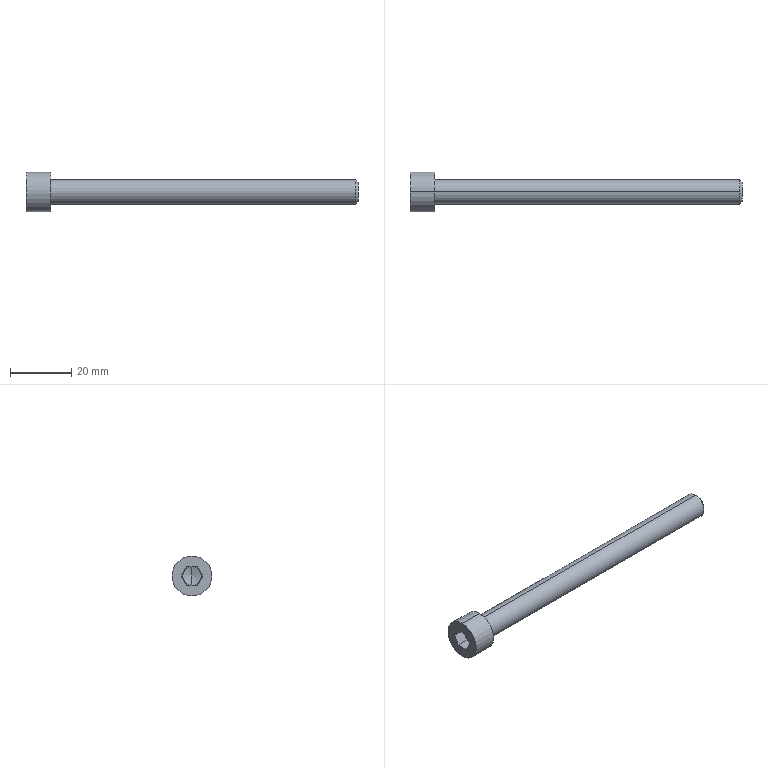Part | STEP file | 0228_301_ACB8-100 | 1 solid | 23 faces | box 108 x 13 x 13 mm | volume 5949 mm3 | plane 15 | cylinder 4 | cone 4 | commonest cylinder face diameters 8 x2 13 x2
STEP:
#1=CARTESIAN_POINT('',(0.,0.,0.));
#2=DIRECTION('',(0.,0.,1.));
#3=DIRECTION('',(1.,0.,0.));
#4=AXIS2_PLACEMENT_3D('',#1,#2,#3);
#5=CARTESIAN_POINT('',(0.,0.,-4.));
#6=VERTEX_POINT('',#5);
#7=CARTESIAN_POINT('',(0.,0.,4.));
#8=VERTEX_POINT('',#7);
#9=CARTESIAN_POINT('',(0.,0.,0.));
#10=DIRECTION('',(1.,0.,0.));
#11=DIRECTION('',(0.,0.,-1.));
#12=AXIS2_PLACEMENT_3D('',#9,#10,#11);
#13=CIRCLE('',#12,4.);
#14=CARTESIAN_POINT('',(49.617,0.,0.));
#15=DIRECTION('',(1.,0.,0.));
#16=DIRECTION('',(0.,0.,-1.));
#17=AXIS2_PLACEMENT_3D('',#14,#15,#16);
#18=CYLINDRICAL_SURFACE('',#17,4.);
#19=CARTESIAN_POINT('',(0.,-49.617));
#20=DIRECTION('',(1.,0.));
#21=VECTOR('',#20,1.);
#22=LINE('',#19,#21);
#23=(GEOMETRIC_REPRESENTATION_CONTEXT(2)PARAMETRIC_REPRESENTATION_CONTEXT()REPRESENTATION_CONTEXT('',''));
#24=DEFINITIONAL_REPRESENTATION('',(#22),#23);
#25=PCURVE('',#18,#24);
#26=CARTESIAN_POINT('',(0.,5.25,0.));
#27=DIRECTION('',(1.,0.,0.));
#28=DIRECTION('',(0.,0.,-1.));
#29=AXIS2_PLACEMENT_3D('',#26,#27,#28);
#30=PLANE('',#29);
#31=CARTESIAN_POINT('',(0.,-5.25));
#32=DIRECTION('',(1.,0.));
#33=AXIS2_PLACEMENT_2D('',#31,#32);
#34=CIRCLE('',#33,4.);
#35=(GEOMETRIC_REPRESENTATION_CONTEXT(2)PARAMETRIC_REPRESENTATION_CONTEXT()REPRESENTATION_CONTEXT('',''));
#36=DEFINITIONAL_REPRESENTATION('',(#34),#35);
#37=PCURVE('',#30,#36);
#38=SURFACE_CURVE('',#13,(#25,#37),.PCURVE_S1.);
#39=EDGE_CURVE('',#6,#8,#38,.T.);
#40=ORIENTED_EDGE('',*,*,#39,.T.);
#41=CARTESIAN_POINT('',(99.233,0.,4.));
#42=VERTEX_POINT('',#41);
#43=CARTESIAN_POINT('',(49.617,0.,4.));
#44=DIRECTION('',(1.,0.,0.));
#45=VECTOR('',#44,1.);
#46=LINE('',#43,#45);
#47=CARTESIAN_POINT('',(3.142,0.));
#48=DIRECTION('',(0.,1.));
#49=VECTOR('',#48,1.);
#50=LINE('',#47,#49);
#51=(GEOMETRIC_REPRESENTATION_CONTEXT(2)PARAMETRIC_REPRESENTATION_CONTEXT()REPRESENTATION_CONTEXT('',''));
#52=DEFINITIONAL_REPRESENTATION('',(#50),#51);
#53=PCURVE('',#18,#52);
#54=CARTESIAN_POINT('',(49.617,0.,0.));
#55=DIRECTION('',(1.,0.,0.));
#56=DIRECTION('',(0.,0.,-1.));
#57=AXIS2_PLACEMENT_3D('',#54,#55,#56);
#58=CYLINDRICAL_SURFACE('',#57,4.);
#59=CARTESIAN_POINT('',(3.142,0.));
#60=DIRECTION('',(0.,1.));
#61=VECTOR('',#60,1.);
#62=LINE('',#59,#61);
#63=(GEOMETRIC_REPRESENTATION_CONTEXT(2)PARAMETRIC_REPRESENTATION_CONTEXT()REPRESENTATION_CONTEXT('',''));
#64=DEFINITIONAL_REPRESENTATION('',(#62),#63);
#65=PCURVE('',#58,#64);
#66=SURFACE_CURVE('',#46,(#53,#65),.PCURVE_S1.);
#67=EDGE_CURVE('',#8,#42,#66,.T.);
#68=ORIENTED_EDGE('',*,*,#67,.T.);
#69=CARTESIAN_POINT('',(99.233,0.,-4.));
#70=VERTEX_POINT('',#69);
#71=CARTESIAN_POINT('',(99.233,0.,0.));
#72=DIRECTION('',(-1.,0.,0.));
#73=DIRECTION('',(0.,0.,-1.));
#74=AXIS2_PLACEMENT_3D('',#71,#72,#73);
#75=CIRCLE('',#74,4.);
#76=CARTESIAN_POINT('',(6.283,49.617));
#77=DIRECTION('',(-1.,0.));
#78=VECTOR('',#77,1.);
#79=LINE('',#76,#78);
#80=(GEOMETRIC_REPRESENTATION_CONTEXT(2)PARAMETRIC_REPRESENTATION_CONTEXT()REPRESENTATION_CONTEXT('',''));
#81=DEFINITIONAL_REPRESENTATION('',(#79),#80);
#82=PCURVE('',#18,#81);
#83=CARTESIAN_POINT('',(99.233,0.,0.));
#84=DIRECTION('',(-1.,0.,0.));
#85=DIRECTION('',(0.,0.,1.));
#86=AXIS2_PLACEMENT_3D('',#83,#84,#85);
#87=CONICAL_SURFACE('',#86,4.,0.7854);
#88=CARTESIAN_POINT('',(-3.142,0.));
#89=DIRECTION('',(1.,0.));
#90=VECTOR('',#89,1.);
#91=LINE('',#88,#90);
#92=(GEOMETRIC_REPRESENTATION_CONTEXT(2)PARAMETRIC_REPRESENTATION_CONTEXT()REPRESENTATION_CONTEXT('',''));
#93=DEFINITIONAL_REPRESENTATION('',(#91),#92);
#94=PCURVE('',#87,#93);
#95=SURFACE_CURVE('',#75,(#82,#94),.PCURVE_S1.);
#96=EDGE_CURVE('',#42,#70,#95,.T.);
#97=ORIENTED_EDGE('',*,*,#96,.T.);
#98=CARTESIAN_POINT('',(49.617,0.,-4.));
#99=DIRECTION('',(1.,0.,0.));
#100=VECTOR('',#99,1.);
#101=LINE('',#98,#100);
#102=CARTESIAN_POINT('',(0.,0.));
#103=DIRECTION('',(0.,1.));
#104=VECTOR('',#103,1.);
#105=LINE('',#102,#104);
#106=(GEOMETRIC_REPRESENTATION_CONTEXT(2)PARAMETRIC_REPRESENTATION_CONTEXT()REPRESENTATION_CONTEXT('',''));
#107=DEFINITIONAL_REPRESENTATION('',(#105),#106);
#108=PCURVE('',#18,#107);
#109=CARTESIAN_POINT('',(6.283,0.));
#110=DIRECTION('',(0.,1.));
#111=VECTOR('',#110,1.);
#112=LINE('',#109,#111);
#113=(GEOMETRIC_REPRESENTATION_CONTEXT(2)PARAMETRIC_REPRESENTATION_CONTEXT()REPRESENTATION_CONTEXT('',''));
#114=DEFINITIONAL_REPRESENTATION('',(#112),#113);
#115=PCURVE('',#58,#114);
#116=SURFACE_CURVE('',#101,(#108,#115),.PCURVE_S1.);
#117=EDGE_CURVE('',#6,#70,#116,.T.);
#118=ORIENTED_EDGE('',*,*,#117,.F.);
#119=EDGE_LOOP('',(#40,#68,#97,#118));
#120=FACE_BOUND('',#119,.T.);
#121=ADVANCED_FACE('',(#120),#18,.T.);
#122=CARTESIAN_POINT('',(100.,0.,3.233));
#123=VERTEX_POINT('',#122);
#124=CARTESIAN_POINT('',(100.,0.,-3.233));
#125=VERTEX_POINT('',#124);
#126=CARTESIAN_POINT('',(100.,0.,0.));
#127=DIRECTION('',(-1.,0.,0.));
#128=DIRECTION('',(0.,0.,1.));
#129=AXIS2_PLACEMENT_3D('',#126,#127,#128);
#130=CIRCLE('',#129,3.233);
#131=CARTESIAN_POINT('',(0.,-0.767));
#132=DIRECTION('',(1.,0.));
#133=VECTOR('',#132,1.);
#134=LINE('',#131,#133);
#135=(GEOMETRIC_REPRESENTATION_CONTEXT(2)PARAMETRIC_REPRESENTATION_CONTEXT()REPRESENTATION_CONTEXT('',''));
#136=DEFINITIONAL_REPRESENTATION('',(#134),#135);
#137=PCURVE('',#87,#136);
#138=CARTESIAN_POINT('',(100.,1.617,0.));
#139=DIRECTION('',(1.,0.,0.));
#140=DIRECTION('',(0.,0.,-1.));
#141=AXIS2_PLACEMENT_3D('',#138,#139,#140);
#142=PLANE('',#141);
#143=CARTESIAN_POINT('',(-3.233,-1.617));
#144=CARTESIAN_POINT('',(-3.233,3.983));
#145=CARTESIAN_POINT('',(1.617,1.183));
#146=CARTESIAN_POINT('',(6.466,-1.617));
#147=CARTESIAN_POINT('',(1.617,-4.416));
#148=CARTESIAN_POINT('',(-3.233,-7.216));
#149=CARTESIAN_POINT('',(-3.233,-1.617));
#150=(BOUNDED_CURVE()B_SPLINE_CURVE(2,(#143,#144,#145,#146,#147,#148,#149),.UNSPECIFIED.,.T.,.F.)B_SPLINE_CURVE_WITH_KNOTS((1,2,2,2,2,1),(-2.094,0.,2.094,4.189,6.283,8.378),.UNSPECIFIED.)CURVE()GEOMETRIC_REPRESENTATION_ITEM()RATIONAL_B_SPLINE_CURVE((1.,0.5,1.,0.5,1.,0.5,1.))REPRESENTATION_ITEM(''));
#151=(GEOMETRIC_REPRESENTATION_CONTEXT(2)PARAMETRIC_REPRESENTATION_CONTEXT()REPRESENTATION_CONTEXT('',''));
#152=DEFINITIONAL_REPRESENTATION('',(#150),#151);
#153=PCURVE('',#142,#152);
#154=SURFACE_CURVE('',#130,(#137,#153),.PCURVE_S1.);
#155=EDGE_CURVE('',#123,#125,#154,.T.);
#156=ORIENTED_EDGE('',*,*,#155,.T.);
#157=CARTESIAN_POINT('',(99.233,0.,-4.));
#158=DIRECTION('',(-0.7071,0.,-0.7071));
#159=VECTOR('',#158,1.);
#160=LINE('',#157,#159);
#161=CARTESIAN_POINT('',(3.142,0.));
#162=DIRECTION('',(0.,1.));
#163=VECTOR('',#162,1.);
#164=LINE('',#161,#163);
#165=(GEOMETRIC_REPRESENTATION_CONTEXT(2)PARAMETRIC_REPRESENTATION_CONTEXT()REPRESENTATION_CONTEXT('',''));
#166=DEFINITIONAL_REPRESENTATION('',(#164),#165);
#167=PCURVE('',#87,#166);
#168=CARTESIAN_POINT('',(99.233,0.,0.));
#169=DIRECTION('',(-1.,0.,0.));
#170=DIRECTION('',(0.,0.,1.));
#171=AXIS2_PLACEMENT_3D('',#168,#169,#170);
#172=CONICAL_SURFACE('',#171,4.,0.7854);
#173=CARTESIAN_POINT('',(3.142,0.));
#174=DIRECTION('',(0.,1.));
#175=VECTOR('',#174,1.);
#176=LINE('',#173,#175);
#177=(GEOMETRIC_REPRESENTATION_CONTEXT(2)PARAMETRIC_REPRESENTATION_CONTEXT()REPRESENTATION_CONTEXT('',''));
#178=DEFINITIONAL_REPRESENTATION('',(#176),#177);
#179=PCURVE('',#172,#178);
#180=SURFACE_CURVE('',#160,(#167,#179),.PCURVE_S1.);
#181=EDGE_CURVE('',#125,#70,#180,.T.);
#182=ORIENTED_EDGE('',*,*,#181,.T.);
#183=ORIENTED_EDGE('',*,*,#96,.F.);
#184=CARTESIAN_POINT('',(99.233,0.,4.));
#185=DIRECTION('',(-0.7071,0.,0.7071));
#186=VECTOR('',#185,1.);
#187=LINE('',#184,#186);
#188=CARTESIAN_POINT('',(0.,0.));
#189=DIRECTION('',(0.,1.));
#190=VECTOR('',#189,1.);
#191=LINE('',#188,#190);
#192=(GEOMETRIC_REPRESENTATION_CONTEXT(2)PARAMETRIC_REPRESENTATION_CONTEXT()REPRESENTATION_CONTEXT('',''));
#193=DEFINITIONAL_REPRESENTATION('',(#191),#192);
#194=PCURVE('',#87,#193);
#195=CARTESIAN_POINT('',(6.283,0.));
#196=DIRECTION('',(0.,1.));
#197=VECTOR('',#196,1.);
#198=LINE('',#195,#197);
#199=(GEOMETRIC_REPRESENTATION_CONTEXT(2)PARAMETRIC_REPRESENTATION_CONTEXT()REPRESENTATION_CONTEXT('',''));
#200=DEFINITIONAL_REPRESENTATION('',(#198),#199);
#201=PCURVE('',#172,#200);
#202=SURFACE_CURVE('',#187,(#194,#201),.PCURVE_S1.);
#203=EDGE_CURVE('',#123,#42,#202,.T.);
#204=ORIENTED_EDGE('',*,*,#203,.F.);
#205=EDGE_LOOP('',(#156,#182,#183,#204));
#206=FACE_BOUND('',#205,.T.);
#207=ADVANCED_FACE('',(#206),#87,.T.);
#208=CARTESIAN_POINT('',(-8.,0.,-6.5));
#209=VERTEX_POINT('',#208);
#210=CARTESIAN_POINT('',(-8.,0.,6.5));
#211=VERTEX_POINT('',#210);
#212=CARTESIAN_POINT('',(-8.,0.,0.));
#213=DIRECTION('',(1.,0.,0.));
#214=DIRECTION('',(0.,0.,-1.));
#215=AXIS2_PLACEMENT_3D('',#212,#213,#214);
#216=CIRCLE('',#215,6.5);
#217=CARTESIAN_POINT('',(-4.,0.,0.));
#218=DIRECTION('',(1.,0.,0.));
#219=DIRECTION('',(0.,0.,-1.));
#220=AXIS2_PLACEMENT_3D('',#217,#218,#219);
#221=CYLINDRICAL_SURFACE('',#220,6.5);
#222=CARTESIAN_POINT('',(0.,-4.));
#223=DIRECTION('',(1.,0.));
#224=VECTOR('',#223,1.);
#225=LINE('',#222,#224);
#226=(GEOMETRIC_REPRESENTATION_CONTEXT(2)PARAMETRIC_REPRESENTATION_CONTEXT()REPRESENTATION_CONTEXT('',''));
#227=DEFINITIONAL_REPRESENTATION('',(#225),#226);
#228=PCURVE('',#221,#227);
#229=CARTESIAN_POINT('',(-8.,3.25,0.));
#230=DIRECTION('',(-1.,0.,0.));
#231=DIRECTION('',(0.,0.,1.));
#232=AXIS2_PLACEMENT_3D('',#229,#230,#231);
#233=PLANE('',#232);
#234=CARTESIAN_POINT('',(-6.5,-3.25));
#235=CARTESIAN_POINT('',(-6.5,8.008));
#236=CARTESIAN_POINT('',(3.25,2.379));
#237=CARTESIAN_POINT('',(13.,-3.25));
#238=CARTESIAN_POINT('',(3.25,-8.879));
#239=CARTESIAN_POINT('',(-6.5,-14.508));
#240=CARTESIAN_POINT('',(-6.5,-3.25));
#241=(BOUNDED_CURVE()B_SPLINE_CURVE(2,(#234,#235,#236,#237,#238,#239,#240),.UNSPECIFIED.,.T.,.F.)B_SPLINE_CURVE_WITH_KNOTS((1,2,2,2,2,1),(-2.094,0.,2.094,4.189,6.283,8.378),.UNSPECIFIED.)CURVE()GEOMETRIC_REPRESENTATION_ITEM()RATIONAL_B_SPLINE_CURVE((1.,0.5,1.,0.5,1.,0.5,1.))REPRESENTATION_ITEM(''));
#242=(GEOMETRIC_REPRESENTATION_CONTEXT(2)PARAMETRIC_REPRESENTATION_CONTEXT()REPRESENTATION_CONTEXT('',''));
#243=DEFINITIONAL_REPRESENTATION('',(#241),#242);
#244=PCURVE('',#233,#243);
#245=SURFACE_CURVE('',#216,(#228,#244),.PCURVE_S1.);
#246=EDGE_CURVE('',#209,#211,#245,.T.);
#247=ORIENTED_EDGE('',*,*,#246,.T.);
#248=CARTESIAN_POINT('',(0.,0.,6.5));
#249=VERTEX_POINT('',#248);
#250=CARTESIAN_POINT('',(-4.,0.,6.5));
#251=DIRECTION('',(1.,0.,0.));
#252=VECTOR('',#251,1.);
#253=LINE('',#250,#252);
#254=CARTESIAN_POINT('',(3.142,0.));
#255=DIRECTION('',(0.,1.));
#256=VECTOR('',#255,1.);
#257=LINE('',#254,#256);
#258=(GEOMETRIC_REPRESENTATION_CONTEXT(2)PARAMETRIC_REPRESENTATION_CONTEXT()REPRESENTATION_CONTEXT('',''));
#259=DEFINITIONAL_REPRESENTATION('',(#257),#258);
#260=PCURVE('',#221,#259);
#261=CARTESIAN_POINT('',(-4.,0.,0.));
#262=DIRECTION('',(1.,0.,0.));
#263=DIRECTION('',(0.,0.,-1.));
#264=AXIS2_PLACEMENT_3D('',#261,#262,#263);
#265=CYLINDRICAL_SURFACE('',#264,6.5);
#266=CARTESIAN_POINT('',(3.142,0.));
#267=DIRECTION('',(0.,1.));
#268=VECTOR('',#267,1.);
#269=LINE('',#266,#268);
#270=(GEOMETRIC_REPRESENTATION_CONTEXT(2)PARAMETRIC_REPRESENTATION_CONTEXT()REPRESENTATION_CONTEXT('',''));
#271=DEFINITIONAL_REPRESENTATION('',(#269),#270);
#272=PCURVE('',#265,#271);
#273=SURFACE_CURVE('',#253,(#260,#272),.PCURVE_S1.);
#274=EDGE_CURVE('',#211,#249,#273,.T.);
#275=ORIENTED_EDGE('',*,*,#274,.T.);
#276=CARTESIAN_POINT('',(0.,0.,-6.5));
#277=VERTEX_POINT('',#276);
#278=CARTESIAN_POINT('',(0.,0.,0.));
#279=DIRECTION('',(1.,0.,0.));
#280=DIRECTION('',(0.,0.,-1.));
#281=AXIS2_PLACEMENT_3D('',#278,#279,#280);
#282=CIRCLE('',#281,6.5);
#283=CARTESIAN_POINT('',(0.,4.));
#284=DIRECTION('',(1.,0.));
#285=VECTOR('',#284,1.);
#286=LINE('',#283,#285);
#287=(GEOMETRIC_REPRESENTATION_CONTEXT(2)PARAMETRIC_REPRESENTATION_CONTEXT()REPRESENTATION_CONTEXT('',''));
#288=DEFINITIONAL_REPRESENTATION('',(#286),#287);
#289=PCURVE('',#221,#288);
#290=CARTESIAN_POINT('',(0.,-5.25));
#291=DIRECTION('',(1.,0.));
#292=AXIS2_PLACEMENT_2D('',#290,#291);
#293=CIRCLE('',#292,6.5);
#294=(GEOMETRIC_REPRESENTATION_CONTEXT(2)PARAMETRIC_REPRESENTATION_CONTEXT()REPRESENTATION_CONTEXT('',''));
#295=DEFINITIONAL_REPRESENTATION('',(#293),#294);
#296=PCURVE('',#30,#295);
#297=SURFACE_CURVE('',#282,(#289,#296),.PCURVE_S1.);
#298=EDGE_CURVE('',#277,#249,#297,.T.);
#299=ORIENTED_EDGE('',*,*,#298,.F.);
#300=CARTESIAN_POINT('',(-4.,0.,-6.5));
#301=DIRECTION('',(1.,0.,0.));
#302=VECTOR('',#301,1.);
#303=LINE('',#300,#302);
#304=CARTESIAN_POINT('',(0.,0.));
#305=DIRECTION('',(0.,1.));
#306=VECTOR('',#305,1.);
#307=LINE('',#304,#306);
#308=(GEOMETRIC_REPRESENTATION_CONTEXT(2)PARAMETRIC_REPRESENTATION_CONTEXT()REPRESENTATION_CONTEXT('',''));
#309=DEFINITIONAL_REPRESENTATION('',(#307),#308);
#310=PCURVE('',#221,#309);
#311=CARTESIAN_POINT('',(6.283,0.));
#312=DIRECTION('',(0.,1.));
#313=VECTOR('',#312,1.);
#314=LINE('',#311,#313);
#315=(GEOMETRIC_REPRESENTATION_CONTEXT(2)PARAMETRIC_REPRESENTATION_CONTEXT()REPRESENTATION_CONTEXT('',''));
#316=DEFINITIONAL_REPRESENTATION('',(#314),#315);
#317=PCURVE('',#265,#316);
#318=SURFACE_CURVE('',#303,(#310,#317),.PCURVE_S1.);
#319=EDGE_CURVE('',#209,#277,#318,.T.);
#320=ORIENTED_EDGE('',*,*,#319,.F.);
#321=EDGE_LOOP('',(#247,#275,#299,#320));
#322=FACE_BOUND('',#321,.T.);
#323=ADVANCED_FACE('',(#322),#221,.T.);
#324=CARTESIAN_POINT('',(-4.,-2.598,1.5));
#325=VERTEX_POINT('',#324);
#326=CARTESIAN_POINT('',(-4.,0.,3.));
#327=VERTEX_POINT('',#326);
#328=CARTESIAN_POINT('',(-4.,0.,0.));
#329=DIRECTION('',(-1.,0.,0.));
#330=DIRECTION('',(0.,0.,1.));
#331=AXIS2_PLACEMENT_3D('',#328,#329,#330);
#332=CIRCLE('',#331,3.);
#333=CARTESIAN_POINT('',(-4.,0.,0.));
#334=DIRECTION('',(-1.,0.,0.));
#335=DIRECTION('',(0.,0.,1.));
#336=AXIS2_PLACEMENT_3D('',#333,#334,#335);
#337=CONICAL_SURFACE('',#336,3.,1.309);
#338=CARTESIAN_POINT('',(0.,0.));
#339=DIRECTION('',(1.,0.));
#340=VECTOR('',#339,1.);
#341=LINE('',#338,#340);
#342=(GEOMETRIC_REPRESENTATION_CONTEXT(2)PARAMETRIC_REPRESENTATION_CONTEXT()REPRESENTATION_CONTEXT('',''));
#343=DEFINITIONAL_REPRESENTATION('',(#341),#342);
#344=PCURVE('',#337,#343);
#345=CARTESIAN_POINT('',(-4.,0.,0.));
#346=DIRECTION('',(1.,0.,0.));
#347=DIRECTION('',(0.,0.,-1.));
#348=AXIS2_PLACEMENT_3D('',#345,#346,#347);
#349=PLANE('',#348);
#350=CARTESIAN_POINT('',(-3.,0.));
#351=CARTESIAN_POINT('',(-3.,5.196));
#352=CARTESIAN_POINT('',(1.5,2.598));
#353=CARTESIAN_POINT('',(6.,0.));
#354=CARTESIAN_POINT('',(1.5,-2.598));
#355=CARTESIAN_POINT('',(-3.,-5.196));
#356=CARTESIAN_POINT('',(-3.,0.));
#357=(BOUNDED_CURVE()B_SPLINE_CURVE(2,(#350,#351,#352,#353,#354,#355,#356),.UNSPECIFIED.,.T.,.F.)B_SPLINE_CURVE_WITH_KNOTS((1,2,2,2,2,1),(-2.094,0.,2.094,4.189,6.283,8.378),.UNSPECIFIED.)CURVE()GEOMETRIC_REPRESENTATION_ITEM()RATIONAL_B_SPLINE_CURVE((1.,0.5,1.,0.5,1.,0.5,1.))REPRESENTATION_ITEM(''));
#358=(GEOMETRIC_REPRESENTATION_CONTEXT(2)PARAMETRIC_REPRESENTATION_CONTEXT()REPRESENTATION_CONTEXT('',''));
#359=DEFINITIONAL_REPRESENTATION('',(#357),#358);
#360=PCURVE('',#349,#359);
#361=SURFACE_CURVE('',#332,(#344,#360),.PCURVE_S1.);
#362=EDGE_CURVE('',#325,#327,#361,.T.);
#363=ORIENTED_EDGE('',*,*,#362,.F.);
#364=CARTESIAN_POINT('',(-4.,-2.598,-1.5));
#365=VERTEX_POINT('',#364);
#366=CARTESIAN_POINT('',(-4.,0.,0.));
#367=DIRECTION('',(1.,0.,0.));
#368=DIRECTION('',(0.,0.,1.));
#369=AXIS2_PLACEMENT_3D('',#366,#367,#368);
#370=CIRCLE('',#369,3.);
#371=CARTESIAN_POINT('',(6.283,0.));
#372=DIRECTION('',(-1.,0.));
#373=VECTOR('',#372,1.);
#374=LINE('',#371,#373);
#375=(GEOMETRIC_REPRESENTATION_CONTEXT(2)PARAMETRIC_REPRESENTATION_CONTEXT()REPRESENTATION_CONTEXT('',''));
#376=DEFINITIONAL_REPRESENTATION('',(#374),#375);
#377=PCURVE('',#337,#376);
#378=CARTESIAN_POINT('',(-4.,0.,0.));
#379=DIRECTION('',(1.,0.,0.));
#380=DIRECTION('',(0.,0.,-1.));
#381=AXIS2_PLACEMENT_3D('',#378,#379,#380);
#382=PLANE('',#381);
#383=CARTESIAN_POINT('',(0.,0.));
#384=DIRECTION('',(-1.,0.));
#385=AXIS2_PLACEMENT_2D('',#383,#384);
#386=CIRCLE('',#385,3.);
#387=(GEOMETRIC_REPRESENTATION_CONTEXT(2)PARAMETRIC_REPRESENTATION_CONTEXT()REPRESENTATION_CONTEXT('',''));
#388=DEFINITIONAL_REPRESENTATION('',(#386),#387);
#389=PCURVE('',#382,#388);
#390=SURFACE_CURVE('',#370,(#377,#389),.PCURVE_S1.);
#391=EDGE_CURVE('',#325,#365,#390,.T.);
#392=ORIENTED_EDGE('',*,*,#391,.T.);
#393=CARTESIAN_POINT('',(-4.,0.,-3.));
#394=VERTEX_POINT('',#393);
#395=CARTESIAN_POINT('',(-4.,0.,0.));
#396=DIRECTION('',(1.,0.,0.));
#397=DIRECTION('',(0.,0.,1.));
#398=AXIS2_PLACEMENT_3D('',#395,#396,#397);
#399=CIRCLE('',#398,3.);
#400=CARTESIAN_POINT('',(6.283,0.));
#401=DIRECTION('',(-1.,0.));
#402=VECTOR('',#401,1.);
#403=LINE('',#400,#402);
#404=(GEOMETRIC_REPRESENTATION_CONTEXT(2)PARAMETRIC_REPRESENTATION_CONTEXT()REPRESENTATION_CONTEXT('',''));
#405=DEFINITIONAL_REPRESENTATION('',(#403),#404);
#406=PCURVE('',#337,#405);
#407=CARTESIAN_POINT('',(-4.,0.,0.));
#408=DIRECTION('',(1.,0.,0.));
#409=DIRECTION('',(0.,0.,-1.));
#410=AXIS2_PLACEMENT_3D('',#407,#408,#409);
#411=PLANE('',#410);
#412=CARTESIAN_POINT('',(0.,0.));
#413=DIRECTION('',(-1.,0.));
#414=AXIS2_PLACEMENT_2D('',#412,#413);
#415=CIRCLE('',#414,3.);
#416=(GEOMETRIC_REPRESENTATION_CONTEXT(2)PARAMETRIC_REPRESENTATION_CONTEXT()REPRESENTATION_CONTEXT('',''));
#417=DEFINITIONAL_REPRESENTATION('',(#415),#416);
#418=PCURVE('',#411,#417);
#419=SURFACE_CURVE('',#399,(#406,#418),.PCURVE_S1.);
#420=EDGE_CURVE('',#365,#394,#419,.T.);
#421=ORIENTED_EDGE('',*,*,#420,.T.);
#422=CARTESIAN_POINT('',(-3.196,0.000000001,0.));
#423=VERTEX_POINT('',#422);
#424=CARTESIAN_POINT('',(-4.,0.,-3.));
#425=DIRECTION('',(-0.2588,0.,-0.9659));
#426=VECTOR('',#425,1.);
#427=LINE('',#424,#426);
#428=CARTESIAN_POINT('',(3.142,0.));
#429=DIRECTION('',(0.,1.));
#430=VECTOR('',#429,1.);
#431=LINE('',#428,#430);
#432=(GEOMETRIC_REPRESENTATION_CONTEXT(2)PARAMETRIC_REPRESENTATION_CONTEXT()REPRESENTATION_CONTEXT('',''));
#433=DEFINITIONAL_REPRESENTATION('',(#431),#432);
#434=PCURVE('',#337,#433);
#435=CARTESIAN_POINT('',(-4.,0.,0.));
#436=DIRECTION('',(-1.,0.,0.));
#437=DIRECTION('',(0.,0.,1.));
#438=AXIS2_PLACEMENT_3D('',#435,#436,#437);
#439=CONICAL_SURFACE('',#438,3.,1.309);
#440=CARTESIAN_POINT('',(3.142,0.));
#441=DIRECTION('',(0.,1.));
#442=VECTOR('',#441,1.);
#443=LINE('',#440,#442);
#444=(GEOMETRIC_REPRESENTATION_CONTEXT(2)PARAMETRIC_REPRESENTATION_CONTEXT()REPRESENTATION_CONTEXT('',''));
#445=DEFINITIONAL_REPRESENTATION('',(#443),#444);
#446=PCURVE('',#439,#445);
#447=SURFACE_CURVE('',#427,(#434,#446),.PCURVE_S1.);
#448=EDGE_CURVE('',#423,#394,#447,.T.);
#449=ORIENTED_EDGE('',*,*,#448,.F.);
#450=CARTESIAN_POINT('',(-4.,0.,3.));
#451=DIRECTION('',(-0.2588,0.,0.9659));
#452=VECTOR('',#451,1.);
#453=LINE('',#450,#452);
#454=CARTESIAN_POINT('',(6.283,0.));
#455=DIRECTION('',(0.,1.));
#456=VECTOR('',#455,1.);
#457=LINE('',#454,#456);
#458=(GEOMETRIC_REPRESENTATION_CONTEXT(2)PARAMETRIC_REPRESENTATION_CONTEXT()REPRESENTATION_CONTEXT('',''));
#459=DEFINITIONAL_REPRESENTATION('',(#457),#458);
#460=PCURVE('',#337,#459);
#461=CARTESIAN_POINT('',(0.,0.));
#462=DIRECTION('',(0.,1.));
#463=VECTOR('',#462,1.);
#464=LINE('',#461,#463);
#465=(GEOMETRIC_REPRESENTATION_CONTEXT(2)PARAMETRIC_REPRESENTATION_CONTEXT()REPRESENTATION_CONTEXT('',''));
#466=DEFINITIONAL_REPRESENTATION('',(#464),#465);
#467=PCURVE('',#439,#466);
#468=SURFACE_CURVE('',#453,(#460,#467),.PCURVE_S1.);
#469=EDGE_CURVE('',#423,#327,#468,.T.);
#470=ORIENTED_EDGE('',*,*,#469,.T.);
#471=EDGE_LOOP('',(#363,#392,#421,#449,#470));
#472=FACE_BOUND('',#471,.F.);
#473=ADVANCED_FACE('',(#472),#337,.F.);
#474=ORIENTED_EDGE('',*,*,#67,.F.);
#475=CARTESIAN_POINT('',(0.,0.,0.));
#476=DIRECTION('',(1.,0.,0.));
#477=DIRECTION('',(0.,0.,-1.));
#478=AXIS2_PLACEMENT_3D('',#475,#476,#477);
#479=CIRCLE('',#478,4.);
#480=CARTESIAN_POINT('',(0.,-49.617));
#481=DIRECTION('',(1.,0.));
#482=VECTOR('',#481,1.);
#483=LINE('',#480,#482);
#484=(GEOMETRIC_REPRESENTATION_CONTEXT(2)PARAMETRIC_REPRESENTATION_CONTEXT()REPRESENTATION_CONTEXT('',''));
#485=DEFINITIONAL_REPRESENTATION('',(#483),#484);
#486=PCURVE('',#58,#485);
#487=CARTESIAN_POINT('',(0.,-5.25));
#488=DIRECTION('',(1.,0.));
#489=AXIS2_PLACEMENT_2D('',#487,#488);
#490=CIRCLE('',#489,4.);
#491=(GEOMETRIC_REPRESENTATION_CONTEXT(2)PARAMETRIC_REPRESENTATION_CONTEXT()REPRESENTATION_CONTEXT('',''));
#492=DEFINITIONAL_REPRESENTATION('',(#490),#491);
#493=PCURVE('',#30,#492);
#494=SURFACE_CURVE('',#479,(#486,#493),.PCURVE_S1.);
#495=EDGE_CURVE('',#8,#6,#494,.T.);
#496=ORIENTED_EDGE('',*,*,#495,.T.);
#497=ORIENTED_EDGE('',*,*,#117,.T.);
#498=CARTESIAN_POINT('',(99.233,0.,0.));
#499=DIRECTION('',(-1.,0.,0.));
#500=DIRECTION('',(0.,0.,-1.));
#501=AXIS2_PLACEMENT_3D('',#498,#499,#500);
#502=CIRCLE('',#501,4.);
#503=CARTESIAN_POINT('',(6.283,49.617));
#504=DIRECTION('',(-1.,0.));
#505=VECTOR('',#504,1.);
#506=LINE('',#503,#505);
#507=(GEOMETRIC_REPRESENTATION_CONTEXT(2)PARAMETRIC_REPRESENTATION_CONTEXT()REPRESENTATION_CONTEXT('',''));
#508=DEFINITIONAL_REPRESENTATION('',(#506),#507);
#509=PCURVE('',#58,#508);
#510=CARTESIAN_POINT('',(3.142,0.));
#511=DIRECTION('',(1.,0.));
#512=VECTOR('',#511,1.);
#513=LINE('',#510,#512);
#514=(GEOMETRIC_REPRESENTATION_CONTEXT(2)PARAMETRIC_REPRESENTATION_CONTEXT()REPRESENTATION_CONTEXT('',''));
#515=DEFINITIONAL_REPRESENTATION('',(#513),#514);
#516=PCURVE('',#172,#515);
#517=SURFACE_CURVE('',#502,(#509,#516),.PCURVE_S1.);
#518=EDGE_CURVE('',#70,#42,#517,.T.);
#519=ORIENTED_EDGE('',*,*,#518,.T.);
#520=EDGE_LOOP('',(#474,#496,#497,#519));
#521=FACE_BOUND('',#520,.T.);
#522=ADVANCED_FACE('',(#521),#58,.T.);
#523=ORIENTED_EDGE('',*,*,#39,.F.);
#524=ORIENTED_EDGE('',*,*,#495,.F.);
#525=EDGE_LOOP('',(#523,#524));
#526=FACE_BOUND('',#525,.T.);
#527=ORIENTED_EDGE('',*,*,#298,.T.);
#528=CARTESIAN_POINT('',(0.,0.,0.));
#529=DIRECTION('',(1.,0.,0.));
#530=DIRECTION('',(0.,0.,-1.));
#531=AXIS2_PLACEMENT_3D('',#528,#529,#530);
#532=CIRCLE('',#531,6.5);
#533=CARTESIAN_POINT('',(0.,-5.25));
#534=DIRECTION('',(1.,0.));
#535=AXIS2_PLACEMENT_2D('',#533,#534);
#536=CIRCLE('',#535,6.5);
#537=(GEOMETRIC_REPRESENTATION_CONTEXT(2)PARAMETRIC_REPRESENTATION_CONTEXT()REPRESENTATION_CONTEXT('',''));
#538=DEFINITIONAL_REPRESENTATION('',(#536),#537);
#539=PCURVE('',#30,#538);
#540=CARTESIAN_POINT('',(0.,4.));
#541=DIRECTION('',(1.,0.));
#542=VECTOR('',#541,1.);
#543=LINE('',#540,#542);
#544=(GEOMETRIC_REPRESENTATION_CONTEXT(2)PARAMETRIC_REPRESENTATION_CONTEXT()REPRESENTATION_CONTEXT('',''));
#545=DEFINITIONAL_REPRESENTATION('',(#543),#544);
#546=PCURVE('',#265,#545);
#547=SURFACE_CURVE('',#532,(#539,#546),.PCURVE_S1.);
#548=EDGE_CURVE('',#249,#277,#547,.T.);
#549=ORIENTED_EDGE('',*,*,#548,.T.);
#550=EDGE_LOOP('',(#527,#549));
#551=FACE_BOUND('',#550,.T.);
#552=ADVANCED_FACE('',(#526,#551),#30,.T.);
#553=ORIENTED_EDGE('',*,*,#181,.F.);
#554=CARTESIAN_POINT('',(100.,0.,0.));
#555=DIRECTION('',(-1.,0.,0.));
#556=DIRECTION('',(0.,0.,1.));
#557=AXIS2_PLACEMENT_3D('',#554,#555,#556);
#558=CIRCLE('',#557,3.233);
#559=CARTESIAN_POINT('',(0.,-0.767));
#560=DIRECTION('',(1.,0.));
#561=VECTOR('',#560,1.);
#562=LINE('',#559,#561);
#563=(GEOMETRIC_REPRESENTATION_CONTEXT(2)PARAMETRIC_REPRESENTATION_CONTEXT()REPRESENTATION_CONTEXT('',''));
#564=DEFINITIONAL_REPRESENTATION('',(#562),#563);
#565=PCURVE('',#172,#564);
#566=CARTESIAN_POINT('',(-3.233,-1.617));
#567=CARTESIAN_POINT('',(-3.233,3.983));
#568=CARTESIAN_POINT('',(1.617,1.183));
#569=CARTESIAN_POINT('',(6.466,-1.617));
#570=CARTESIAN_POINT('',(1.617,-4.416));
#571=CARTESIAN_POINT('',(-3.233,-7.216));
#572=CARTESIAN_POINT('',(-3.233,-1.617));
#573=(BOUNDED_CURVE()B_SPLINE_CURVE(2,(#566,#567,#568,#569,#570,#571,#572),.UNSPECIFIED.,.T.,.F.)B_SPLINE_CURVE_WITH_KNOTS((1,2,2,2,2,1),(-2.094,0.,2.094,4.189,6.283,8.378),.UNSPECIFIED.)CURVE()GEOMETRIC_REPRESENTATION_ITEM()RATIONAL_B_SPLINE_CURVE((1.,0.5,1.,0.5,1.,0.5,1.))REPRESENTATION_ITEM(''));
#574=(GEOMETRIC_REPRESENTATION_CONTEXT(2)PARAMETRIC_REPRESENTATION_CONTEXT()REPRESENTATION_CONTEXT('',''));
#575=DEFINITIONAL_REPRESENTATION('',(#573),#574);
#576=PCURVE('',#142,#575);
#577=SURFACE_CURVE('',#558,(#565,#576),.PCURVE_S1.);
#578=EDGE_CURVE('',#125,#123,#577,.T.);
#579=ORIENTED_EDGE('',*,*,#578,.T.);
#580=ORIENTED_EDGE('',*,*,#203,.T.);
#581=ORIENTED_EDGE('',*,*,#518,.F.);
#582=EDGE_LOOP('',(#553,#579,#580,#581));
#583=FACE_BOUND('',#582,.T.);
#584=ADVANCED_FACE('',(#583),#172,.T.);
#585=ORIENTED_EDGE('',*,*,#274,.F.);
#586=CARTESIAN_POINT('',(-8.,0.,0.));
#587=DIRECTION('',(1.,0.,0.));
#588=DIRECTION('',(0.,0.,-1.));
#589=AXIS2_PLACEMENT_3D('',#586,#587,#588);
#590=CIRCLE('',#589,6.5);
#591=CARTESIAN_POINT('',(0.,-4.));
#592=DIRECTION('',(1.,0.));
#593=VECTOR('',#592,1.);
#594=LINE('',#591,#593);
#595=(GEOMETRIC_REPRESENTATION_CONTEXT(2)PARAMETRIC_REPRESENTATION_CONTEXT()REPRESENTATION_CONTEXT('',''));
#596=DEFINITIONAL_REPRESENTATION('',(#594),#595);
#597=PCURVE('',#265,#596);
#598=CARTESIAN_POINT('',(-6.5,-3.25));
#599=CARTESIAN_POINT('',(-6.5,8.008));
#600=CARTESIAN_POINT('',(3.25,2.379));
#601=CARTESIAN_POINT('',(13.,-3.25));
#602=CARTESIAN_POINT('',(3.25,-8.879));
#603=CARTESIAN_POINT('',(-6.5,-14.508));
#604=CARTESIAN_POINT('',(-6.5,-3.25));
#605=(BOUNDED_CURVE()B_SPLINE_CURVE(2,(#598,#599,#600,#601,#602,#603,#604),.UNSPECIFIED.,.T.,.F.)B_SPLINE_CURVE_WITH_KNOTS((1,2,2,2,2,1),(-2.094,0.,2.094,4.189,6.283,8.378),.UNSPECIFIED.)CURVE()GEOMETRIC_REPRESENTATION_ITEM()RATIONAL_B_SPLINE_CURVE((1.,0.5,1.,0.5,1.,0.5,1.))REPRESENTATION_ITEM(''));
#606=(GEOMETRIC_REPRESENTATION_CONTEXT(2)PARAMETRIC_REPRESENTATION_CONTEXT()REPRESENTATION_CONTEXT('',''));
#607=DEFINITIONAL_REPRESENTATION('',(#605),#606);
#608=PCURVE('',#233,#607);
#609=SURFACE_CURVE('',#590,(#597,#608),.PCURVE_S1.);
#610=EDGE_CURVE('',#211,#209,#609,.T.);
#611=ORIENTED_EDGE('',*,*,#610,.T.);
#612=ORIENTED_EDGE('',*,*,#319,.T.);
#613=ORIENTED_EDGE('',*,*,#548,.F.);
#614=EDGE_LOOP('',(#585,#611,#612,#613));
#615=FACE_BOUND('',#614,.T.);
#616=ADVANCED_FACE('',(#615),#265,.T.);
#617=ORIENTED_EDGE('',*,*,#155,.F.);
#618=ORIENTED_EDGE('',*,*,#578,.F.);
#619=EDGE_LOOP('',(#617,#618));
#620=FACE_BOUND('',#619,.T.);
#621=ADVANCED_FACE('',(#620),#142,.T.);
#622=ORIENTED_EDGE('',*,*,#246,.F.);
#623=ORIENTED_EDGE('',*,*,#610,.F.);
#624=EDGE_LOOP('',(#622,#623));
#625=FACE_BOUND('',#624,.T.);
#626=CARTESIAN_POINT('',(-8.,1.732,-3.));
#627=VERTEX_POINT('',#626);
#628=CARTESIAN_POINT('',(-8.,3.464,0.));
#629=VERTEX_POINT('',#628);
#630=CARTESIAN_POINT('',(-8.,1.732,-3.));
#631=DIRECTION('',(0.,0.5,0.866));
#632=VECTOR('',#631,1.);
#633=LINE('',#630,#632);
#634=CARTESIAN_POINT('',(-3.,-1.518));
#635=DIRECTION('',(0.866,0.5));
#636=VECTOR('',#635,1.);
#637=LINE('',#634,#636);
#638=(GEOMETRIC_REPRESENTATION_CONTEXT(2)PARAMETRIC_REPRESENTATION_CONTEXT()REPRESENTATION_CONTEXT('',''));
#639=DEFINITIONAL_REPRESENTATION('',(#637),#638);
#640=PCURVE('',#233,#639);
#641=CARTESIAN_POINT('',(-8.,3.464,0.));
#642=DIRECTION('',(0.,0.866,-0.5));
#643=DIRECTION('',(0.,0.5,0.866));
#644=AXIS2_PLACEMENT_3D('',#641,#642,#643);
#645=PLANE('',#644);
#646=CARTESIAN_POINT('',(-3.464,0.));
#647=DIRECTION('',(1.,0.));
#648=VECTOR('',#647,1.);
#649=LINE('',#646,#648);
#650=(GEOMETRIC_REPRESENTATION_CONTEXT(2)PARAMETRIC_REPRESENTATION_CONTEXT()REPRESENTATION_CONTEXT('',''));
#651=DEFINITIONAL_REPRESENTATION('',(#649),#650);
#652=PCURVE('',#645,#651);
#653=SURFACE_CURVE('',#633,(#640,#652),.PCURVE_S1.);
#654=EDGE_CURVE('',#627,#629,#653,.T.);
#655=ORIENTED_EDGE('',*,*,#654,.T.);
#656=CARTESIAN_POINT('',(-8.,1.732,3.));
#657=VERTEX_POINT('',#656);
#658=CARTESIAN_POINT('',(-8.,3.464,0.));
#659=DIRECTION('',(0.,-0.5,0.866));
#660=VECTOR('',#659,1.);
#661=LINE('',#658,#660);
#662=CARTESIAN_POINT('',(0.,0.2141));
#663=DIRECTION('',(0.866,-0.5));
#664=VECTOR('',#663,1.);
#665=LINE('',#662,#664);
#666=(GEOMETRIC_REPRESENTATION_CONTEXT(2)PARAMETRIC_REPRESENTATION_CONTEXT()REPRESENTATION_CONTEXT('',''));
#667=DEFINITIONAL_REPRESENTATION('',(#665),#666);
#668=PCURVE('',#233,#667);
#669=CARTESIAN_POINT('',(-8.,1.732,3.));
#670=DIRECTION('',(0.,0.866,0.5));
#671=DIRECTION('',(0.,-0.5,0.866));
#672=AXIS2_PLACEMENT_3D('',#669,#670,#671);
#673=PLANE('',#672);
#674=CARTESIAN_POINT('',(-3.464,0.));
#675=DIRECTION('',(1.,0.));
#676=VECTOR('',#675,1.);
#677=LINE('',#674,#676);
#678=(GEOMETRIC_REPRESENTATION_CONTEXT(2)PARAMETRIC_REPRESENTATION_CONTEXT()REPRESENTATION_CONTEXT('',''));
#679=DEFINITIONAL_REPRESENTATION('',(#677),#678);
#680=PCURVE('',#673,#679);
#681=SURFACE_CURVE('',#661,(#668,#680),.PCURVE_S1.);
#682=EDGE_CURVE('',#629,#657,#681,.T.);
#683=ORIENTED_EDGE('',*,*,#682,.T.);
#684=CARTESIAN_POINT('',(-8.,-1.732,3.));
#685=VERTEX_POINT('',#684);
#686=CARTESIAN_POINT('',(-8.,3.25,3.));
#687=DIRECTION('',(0.,-1.,0.));
#688=VECTOR('',#687,1.);
#689=LINE('',#686,#688);
#690=CARTESIAN_POINT('',(3.,0.));
#691=DIRECTION('',(0.,-1.));
#692=VECTOR('',#691,1.);
#693=LINE('',#690,#692);
#694=(GEOMETRIC_REPRESENTATION_CONTEXT(2)PARAMETRIC_REPRESENTATION_CONTEXT()REPRESENTATION_CONTEXT('',''));
#695=DEFINITIONAL_REPRESENTATION('',(#693),#694);
#696=PCURVE('',#233,#695);
#697=CARTESIAN_POINT('',(-8.,-1.732,3.));
#698=DIRECTION('',(0.,0.,1.));
#699=DIRECTION('',(1.,0.,0.));
#700=AXIS2_PLACEMENT_3D('',#697,#698,#699);
#701=PLANE('',#700);
#702=CARTESIAN_POINT('',(0.,4.982));
#703=DIRECTION('',(0.,-1.));
#704=VECTOR('',#703,1.);
#705=LINE('',#702,#704);
#706=(GEOMETRIC_REPRESENTATION_CONTEXT(2)PARAMETRIC_REPRESENTATION_CONTEXT()REPRESENTATION_CONTEXT('',''));
#707=DEFINITIONAL_REPRESENTATION('',(#705),#706);
#708=PCURVE('',#701,#707);
#709=SURFACE_CURVE('',#689,(#696,#708),.PCURVE_S1.);
#710=EDGE_CURVE('',#657,#685,#709,.T.);
#711=ORIENTED_EDGE('',*,*,#710,.T.);
#712=CARTESIAN_POINT('',(-8.,-3.464,0.));
#713=VERTEX_POINT('',#712);
#714=CARTESIAN_POINT('',(-8.,-1.732,3.));
#715=DIRECTION('',(0.,-0.5,-0.866));
#716=VECTOR('',#715,1.);
#717=LINE('',#714,#716);
#718=CARTESIAN_POINT('',(3.,-4.982));
#719=DIRECTION('',(-0.866,-0.5));
#720=VECTOR('',#719,1.);
#721=LINE('',#718,#720);
#722=(GEOMETRIC_REPRESENTATION_CONTEXT(2)PARAMETRIC_REPRESENTATION_CONTEXT()REPRESENTATION_CONTEXT('',''));
#723=DEFINITIONAL_REPRESENTATION('',(#721),#722);
#724=PCURVE('',#233,#723);
#725=CARTESIAN_POINT('',(-8.,-3.464,0.));
#726=DIRECTION('',(0.,-0.866,0.5));
#727=DIRECTION('',(0.,-0.5,-0.866));
#728=AXIS2_PLACEMENT_3D('',#725,#726,#727);
#729=PLANE('',#728);
#730=CARTESIAN_POINT('',(-3.464,0.));
#731=DIRECTION('',(1.,0.));
#732=VECTOR('',#731,1.);
#733=LINE('',#730,#732);
#734=(GEOMETRIC_REPRESENTATION_CONTEXT(2)PARAMETRIC_REPRESENTATION_CONTEXT()REPRESENTATION_CONTEXT('',''));
#735=DEFINITIONAL_REPRESENTATION('',(#733),#734);
#736=PCURVE('',#729,#735);
#737=SURFACE_CURVE('',#717,(#724,#736),.PCURVE_S1.);
#738=EDGE_CURVE('',#685,#713,#737,.T.);
#739=ORIENTED_EDGE('',*,*,#738,.T.);
#740=CARTESIAN_POINT('',(-8.,-1.732,-3.));
#741=VERTEX_POINT('',#740);
#742=CARTESIAN_POINT('',(-8.,-3.464,0.));
#743=DIRECTION('',(0.,0.5,-0.866));
#744=VECTOR('',#743,1.);
#745=LINE('',#742,#744);
#746=CARTESIAN_POINT('',(0.,-6.714));
#747=DIRECTION('',(-0.866,0.5));
#748=VECTOR('',#747,1.);
#749=LINE('',#746,#748);
#750=(GEOMETRIC_REPRESENTATION_CONTEXT(2)PARAMETRIC_REPRESENTATION_CONTEXT()REPRESENTATION_CONTEXT('',''));
#751=DEFINITIONAL_REPRESENTATION('',(#749),#750);
#752=PCURVE('',#233,#751);
#753=CARTESIAN_POINT('',(-8.,-1.732,-3.));
#754=DIRECTION('',(0.,-0.866,-0.5));
#755=DIRECTION('',(0.,0.5,-0.866));
#756=AXIS2_PLACEMENT_3D('',#753,#754,#755);
#757=PLANE('',#756);
#758=CARTESIAN_POINT('',(-3.464,0.));
#759=DIRECTION('',(1.,0.));
#760=VECTOR('',#759,1.);
#761=LINE('',#758,#760);
#762=(GEOMETRIC_REPRESENTATION_CONTEXT(2)PARAMETRIC_REPRESENTATION_CONTEXT()REPRESENTATION_CONTEXT('',''));
#763=DEFINITIONAL_REPRESENTATION('',(#761),#762);
#764=PCURVE('',#757,#763);
#765=SURFACE_CURVE('',#745,(#752,#764),.PCURVE_S1.);
#766=EDGE_CURVE('',#713,#741,#765,.T.);
#767=ORIENTED_EDGE('',*,*,#766,.T.);
#768=CARTESIAN_POINT('',(-8.,3.25,-3.));
#769=DIRECTION('',(0.,1.,0.));
#770=VECTOR('',#769,1.);
#771=LINE('',#768,#770);
#772=CARTESIAN_POINT('',(-3.,0.));
#773=DIRECTION('',(0.,1.));
#774=VECTOR('',#773,1.);
#775=LINE('',#772,#774);
#776=(GEOMETRIC_REPRESENTATION_CONTEXT(2)PARAMETRIC_REPRESENTATION_CONTEXT()REPRESENTATION_CONTEXT('',''));
#777=DEFINITIONAL_REPRESENTATION('',(#775),#776);
#778=PCURVE('',#233,#777);
#779=CARTESIAN_POINT('',(-8.,1.732,-3.));
#780=DIRECTION('',(0.,0.,-1.));
#781=DIRECTION('',(-1.,0.,0.));
#782=AXIS2_PLACEMENT_3D('',#779,#780,#781);
#783=PLANE('',#782);
#784=CARTESIAN_POINT('',(0.,1.518));
#785=DIRECTION('',(0.,1.));
#786=VECTOR('',#785,1.);
#787=LINE('',#784,#786);
#788=(GEOMETRIC_REPRESENTATION_CONTEXT(2)PARAMETRIC_REPRESENTATION_CONTEXT()REPRESENTATION_CONTEXT('',''));
#789=DEFINITIONAL_REPRESENTATION('',(#787),#788);
#790=PCURVE('',#783,#789);
#791=SURFACE_CURVE('',#771,(#778,#790),.PCURVE_S1.);
#792=EDGE_CURVE('',#741,#627,#791,.T.);
#793=ORIENTED_EDGE('',*,*,#792,.T.);
#794=EDGE_LOOP('',(#655,#683,#711,#739,#767,#793));
#795=FACE_BOUND('',#794,.T.);
#796=ADVANCED_FACE('',(#625,#795),#233,.T.);
#797=CARTESIAN_POINT('',(-4.,3.464,0.));
#798=VERTEX_POINT('',#797);
#799=CARTESIAN_POINT('',(-8.,3.464,0.));
#800=DIRECTION('',(-1.,0.,0.));
#801=VECTOR('',#800,1.);
#802=LINE('',#799,#801);
#803=CARTESIAN_POINT('',(-3.464,0.));
#804=DIRECTION('',(0.,-1.));
#805=VECTOR('',#804,1.);
#806=LINE('',#803,#805);
#807=(GEOMETRIC_REPRESENTATION_CONTEXT(2)PARAMETRIC_REPRESENTATION_CONTEXT()REPRESENTATION_CONTEXT('',''));
#808=DEFINITIONAL_REPRESENTATION('',(#806),#807);
#809=PCURVE('',#673,#808);
#810=CARTESIAN_POINT('',(0.,0.));
#811=DIRECTION('',(0.,-1.));
#812=VECTOR('',#811,1.);
#813=LINE('',#810,#812);
#814=(GEOMETRIC_REPRESENTATION_CONTEXT(2)PARAMETRIC_REPRESENTATION_CONTEXT()REPRESENTATION_CONTEXT('',''));
#815=DEFINITIONAL_REPRESENTATION('',(#813),#814);
#816=PCURVE('',#645,#815);
#817=SURFACE_CURVE('',#802,(#809,#816),.PCURVE_S1.);
#818=EDGE_CURVE('',#798,#629,#817,.T.);
#819=ORIENTED_EDGE('',*,*,#818,.F.);
#820=CARTESIAN_POINT('',(-4.,2.598,1.5));
#821=VERTEX_POINT('',#820);
#822=CARTESIAN_POINT('',(-4.,1.732,3.));
#823=DIRECTION('',(0.,0.5,-0.866));
#824=VECTOR('',#823,1.);
#825=LINE('',#822,#824);
#826=CARTESIAN_POINT('',(0.,4.));
#827=DIRECTION('',(-1.,0.));
#828=VECTOR('',#827,1.);
#829=LINE('',#826,#828);
#830=(GEOMETRIC_REPRESENTATION_CONTEXT(2)PARAMETRIC_REPRESENTATION_CONTEXT()REPRESENTATION_CONTEXT('',''));
#831=DEFINITIONAL_REPRESENTATION('',(#829),#830);
#832=PCURVE('',#673,#831);
#833=CARTESIAN_POINT('',(-4.,0.,0.));
#834=DIRECTION('',(1.,0.,0.));
#835=DIRECTION('',(0.,0.,-1.));
#836=AXIS2_PLACEMENT_3D('',#833,#834,#835);
#837=PLANE('',#836);
#838=CARTESIAN_POINT('',(-3.,1.732));
#839=DIRECTION('',(0.866,0.5));
#840=VECTOR('',#839,1.);
#841=LINE('',#838,#840);
#842=(GEOMETRIC_REPRESENTATION_CONTEXT(2)PARAMETRIC_REPRESENTATION_CONTEXT()REPRESENTATION_CONTEXT('',''));
#843=DEFINITIONAL_REPRESENTATION('',(#841),#842);
#844=PCURVE('',#837,#843);
#845=SURFACE_CURVE('',#825,(#832,#844),.PCURVE_S1.);
#846=EDGE_CURVE('',#821,#798,#845,.T.);
#847=ORIENTED_EDGE('',*,*,#846,.F.);
#848=CARTESIAN_POINT('',(-4.,1.732,3.));
#849=VERTEX_POINT('',#848);
#850=CARTESIAN_POINT('',(-4.,2.598,1.5));
#851=DIRECTION('',(0.,-0.5,0.866));
#852=VECTOR('',#851,1.);
#853=LINE('',#850,#852);
#854=CARTESIAN_POINT('',(-1.732,4.));
#855=DIRECTION('',(1.,0.));
#856=VECTOR('',#855,1.);
#857=LINE('',#854,#856);
#858=(GEOMETRIC_REPRESENTATION_CONTEXT(2)PARAMETRIC_REPRESENTATION_CONTEXT()REPRESENTATION_CONTEXT('',''));
#859=DEFINITIONAL_REPRESENTATION('',(#857),#858);
#860=PCURVE('',#673,#859);
#861=CARTESIAN_POINT('',(-4.,0.,0.));
#862=DIRECTION('',(1.,0.,0.));
#863=DIRECTION('',(0.,0.,-1.));
#864=AXIS2_PLACEMENT_3D('',#861,#862,#863);
#865=PLANE('',#864);
#866=CARTESIAN_POINT('',(-1.5,2.598));
#867=DIRECTION('',(-0.866,-0.5));
#868=VECTOR('',#867,1.);
#869=LINE('',#866,#868);
#870=(GEOMETRIC_REPRESENTATION_CONTEXT(2)PARAMETRIC_REPRESENTATION_CONTEXT()REPRESENTATION_CONTEXT('',''));
#871=DEFINITIONAL_REPRESENTATION('',(#869),#870);
#872=PCURVE('',#865,#871);
#873=SURFACE_CURVE('',#853,(#860,#872),.PCURVE_S1.);
#874=EDGE_CURVE('',#821,#849,#873,.T.);
#875=ORIENTED_EDGE('',*,*,#874,.T.);
#876=CARTESIAN_POINT('',(-8.,1.732,3.));
#877=DIRECTION('',(1.,0.,0.));
#878=VECTOR('',#877,1.);
#879=LINE('',#876,#878);
#880=CARTESIAN_POINT('',(0.,0.));
#881=DIRECTION('',(0.,1.));
#882=VECTOR('',#881,1.);
#883=LINE('',#880,#882);
#884=(GEOMETRIC_REPRESENTATION_CONTEXT(2)PARAMETRIC_REPRESENTATION_CONTEXT()REPRESENTATION_CONTEXT('',''));
#885=DEFINITIONAL_REPRESENTATION('',(#883),#884);
#886=PCURVE('',#673,#885);
#887=CARTESIAN_POINT('',(0.,3.464));
#888=DIRECTION('',(1.,0.));
#889=VECTOR('',#888,1.);
#890=LINE('',#887,#889);
#891=(GEOMETRIC_REPRESENTATION_CONTEXT(2)PARAMETRIC_REPRESENTATION_CONTEXT()REPRESENTATION_CONTEXT('',''));
#892=DEFINITIONAL_REPRESENTATION('',(#890),#891);
#893=PCURVE('',#701,#892);
#894=SURFACE_CURVE('',#879,(#886,#893),.PCURVE_S1.);
#895=EDGE_CURVE('',#657,#849,#894,.T.);
#896=ORIENTED_EDGE('',*,*,#895,.F.);
#897=ORIENTED_EDGE('',*,*,#682,.F.);
#898=EDGE_LOOP('',(#819,#847,#875,#896,#897));
#899=FACE_BOUND('',#898,.T.);
#900=ADVANCED_FACE('',(#899),#673,.F.);
#901=CARTESIAN_POINT('',(-4.,1.732,-3.));
#902=VERTEX_POINT('',#901);
#903=CARTESIAN_POINT('',(-8.,1.732,-3.));
#904=DIRECTION('',(-1.,0.,0.));
#905=VECTOR('',#904,1.);
#906=LINE('',#903,#905);
#907=CARTESIAN_POINT('',(-3.464,0.));
#908=DIRECTION('',(0.,-1.));
#909=VECTOR('',#908,1.);
#910=LINE('',#907,#909);
#911=(GEOMETRIC_REPRESENTATION_CONTEXT(2)PARAMETRIC_REPRESENTATION_CONTEXT()REPRESENTATION_CONTEXT('',''));
#912=DEFINITIONAL_REPRESENTATION('',(#910),#911);
#913=PCURVE('',#645,#912);
#914=CARTESIAN_POINT('',(0.,0.));
#915=DIRECTION('',(1.,0.));
#916=VECTOR('',#915,1.);
#917=LINE('',#914,#916);
#918=(GEOMETRIC_REPRESENTATION_CONTEXT(2)PARAMETRIC_REPRESENTATION_CONTEXT()REPRESENTATION_CONTEXT('',''));
#919=DEFINITIONAL_REPRESENTATION('',(#917),#918);
#920=PCURVE('',#783,#919);
#921=SURFACE_CURVE('',#906,(#913,#920),.PCURVE_S1.);
#922=EDGE_CURVE('',#902,#627,#921,.T.);
#923=ORIENTED_EDGE('',*,*,#922,.F.);
#924=CARTESIAN_POINT('',(-4.,2.598,-1.5));
#925=VERTEX_POINT('',#924);
#926=CARTESIAN_POINT('',(-4.,1.732,-3.));
#927=DIRECTION('',(0.,0.5,0.866));
#928=VECTOR('',#927,1.);
#929=LINE('',#926,#928);
#930=CARTESIAN_POINT('',(-3.464,4.));
#931=DIRECTION('',(1.,0.));
#932=VECTOR('',#931,1.);
#933=LINE('',#930,#932);
#934=(GEOMETRIC_REPRESENTATION_CONTEXT(2)PARAMETRIC_REPRESENTATION_CONTEXT()REPRESENTATION_CONTEXT('',''));
#935=DEFINITIONAL_REPRESENTATION('',(#933),#934);
#936=PCURVE('',#645,#935);
#937=CARTESIAN_POINT('',(-4.,0.,0.));
#938=DIRECTION('',(1.,0.,0.));
#939=DIRECTION('',(0.,0.,-1.));
#940=AXIS2_PLACEMENT_3D('',#937,#938,#939);
#941=PLANE('',#940);
#942=CARTESIAN_POINT('',(3.,1.732));
#943=DIRECTION('',(-0.866,0.5));
#944=VECTOR('',#943,1.);
#945=LINE('',#942,#944);
#946=(GEOMETRIC_REPRESENTATION_CONTEXT(2)PARAMETRIC_REPRESENTATION_CONTEXT()REPRESENTATION_CONTEXT('',''));
#947=DEFINITIONAL_REPRESENTATION('',(#945),#946);
#948=PCURVE('',#941,#947);
#949=SURFACE_CURVE('',#929,(#936,#948),.PCURVE_S1.);
#950=EDGE_CURVE('',#902,#925,#949,.T.);
#951=ORIENTED_EDGE('',*,*,#950,.T.);
#952=CARTESIAN_POINT('',(-4.,3.464,0.));
#953=DIRECTION('',(0.,-0.5,-0.866));
#954=VECTOR('',#953,1.);
#955=LINE('',#952,#954);
#956=CARTESIAN_POINT('',(0.,4.));
#957=DIRECTION('',(-1.,0.));
#958=VECTOR('',#957,1.);
#959=LINE('',#956,#958);
#960=(GEOMETRIC_REPRESENTATION_CONTEXT(2)PARAMETRIC_REPRESENTATION_CONTEXT()REPRESENTATION_CONTEXT('',''));
#961=DEFINITIONAL_REPRESENTATION('',(#959),#960);
#962=PCURVE('',#645,#961);
#963=CARTESIAN_POINT('',(0.,3.464));
#964=DIRECTION('',(0.866,-0.5));
#965=VECTOR('',#964,1.);
#966=LINE('',#963,#965);
#967=(GEOMETRIC_REPRESENTATION_CONTEXT(2)PARAMETRIC_REPRESENTATION_CONTEXT()REPRESENTATION_CONTEXT('',''));
#968=DEFINITIONAL_REPRESENTATION('',(#966),#967);
#969=PCURVE('',#837,#968);
#970=SURFACE_CURVE('',#955,(#962,#969),.PCURVE_S1.);
#971=EDGE_CURVE('',#798,#925,#970,.T.);
#972=ORIENTED_EDGE('',*,*,#971,.F.);
#973=ORIENTED_EDGE('',*,*,#818,.T.);
#974=ORIENTED_EDGE('',*,*,#654,.F.);
#975=EDGE_LOOP('',(#923,#951,#972,#973,#974));
#976=FACE_BOUND('',#975,.T.);
#977=ADVANCED_FACE('',(#976),#645,.F.);
#978=CARTESIAN_POINT('',(-4.,-1.732,-3.));
#979=VERTEX_POINT('',#978);
#980=CARTESIAN_POINT('',(-8.,-1.732,-3.));
#981=DIRECTION('',(-1.,0.,0.));
#982=VECTOR('',#981,1.);
#983=LINE('',#980,#982);
#984=CARTESIAN_POINT('',(0.,-3.464));
#985=DIRECTION('',(1.,0.));
#986=VECTOR('',#985,1.);
#987=LINE('',#984,#986);
#988=(GEOMETRIC_REPRESENTATION_CONTEXT(2)PARAMETRIC_REPRESENTATION_CONTEXT()REPRESENTATION_CONTEXT('',''));
#989=DEFINITIONAL_REPRESENTATION('',(#987),#988);
#990=PCURVE('',#783,#989);
#991=CARTESIAN_POINT('',(0.,0.));
#992=DIRECTION('',(0.,-1.));
#993=VECTOR('',#992,1.);
#994=LINE('',#991,#993);
#995=(GEOMETRIC_REPRESENTATION_CONTEXT(2)PARAMETRIC_REPRESENTATION_CONTEXT()REPRESENTATION_CONTEXT('',''));
#996=DEFINITIONAL_REPRESENTATION('',(#994),#995);
#997=PCURVE('',#757,#996);
#998=SURFACE_CURVE('',#983,(#990,#997),.PCURVE_S1.);
#999=EDGE_CURVE('',#979,#741,#998,.T.);
#1000=ORIENTED_EDGE('',*,*,#999,.F.);
#1001=CARTESIAN_POINT('',(-4.,0.,-3.));
#1002=DIRECTION('',(0.,1.,0.));
#1003=VECTOR('',#1002,1.);
#1004=LINE('',#1001,#1003);
#1005=CARTESIAN_POINT('',(-4.,-1.732));
#1006=DIRECTION('',(0.,1.));
#1007=VECTOR('',#1006,1.);
#1008=LINE('',#1005,#1007);
#1009=(GEOMETRIC_REPRESENTATION_CONTEXT(2)PARAMETRIC_REPRESENTATION_CONTEXT()REPRESENTATION_CONTEXT('',''));
#1010=DEFINITIONAL_REPRESENTATION('',(#1008),#1009);
#1011=PCURVE('',#783,#1010);
#1012=CARTESIAN_POINT('',(3.,0.));
#1013=DIRECTION('',(0.,1.));
#1014=VECTOR('',#1013,1.);
#1015=LINE('',#1012,#1014);
#1016=(GEOMETRIC_REPRESENTATION_CONTEXT(2)PARAMETRIC_REPRESENTATION_CONTEXT()REPRESENTATION_CONTEXT('',''));
#1017=DEFINITIONAL_REPRESENTATION('',(#1015),#1016);
#1018=PCURVE('',#411,#1017);
#1019=SURFACE_CURVE('',#1004,(#1011,#1018),.PCURVE_S1.);
#1020=EDGE_CURVE('',#979,#394,#1019,.T.);
#1021=ORIENTED_EDGE('',*,*,#1020,.T.);
#1022=CARTESIAN_POINT('',(-4.,0.,-3.));
#1023=DIRECTION('',(0.,1.,0.));
#1024=VECTOR('',#1023,1.);
#1025=LINE('',#1022,#1024);
#1026=CARTESIAN_POINT('',(-4.,-1.732));
#1027=DIRECTION('',(0.,1.));
#1028=VECTOR('',#1027,1.);
#1029=LINE('',#1026,#1028);
#1030=(GEOMETRIC_REPRESENTATION_CONTEXT(2)PARAMETRIC_REPRESENTATION_CONTEXT()REPRESENTATION_CONTEXT('',''));
#1031=DEFINITIONAL_REPRESENTATION('',(#1029),#1030);
#1032=PCURVE('',#783,#1031);
#1033=CARTESIAN_POINT('',(3.,0.));
#1034=DIRECTION('',(0.,1.));
#1035=VECTOR('',#1034,1.);
#1036=LINE('',#1033,#1035);
#1037=(GEOMETRIC_REPRESENTATION_CONTEXT(2)PARAMETRIC_REPRESENTATION_CONTEXT()REPRESENTATION_CONTEXT('',''));
#1038=DEFINITIONAL_REPRESENTATION('',(#1036),#1037);
#1039=PCURVE('',#941,#1038);
#1040=SURFACE_CURVE('',#1025,(#1032,#1039),.PCURVE_S1.);
#1041=EDGE_CURVE('',#394,#902,#1040,.T.);
#1042=ORIENTED_EDGE('',*,*,#1041,.T.);
#1043=ORIENTED_EDGE('',*,*,#922,.T.);
#1044=ORIENTED_EDGE('',*,*,#792,.F.);
#1045=EDGE_LOOP('',(#1000,#1021,#1042,#1043,#1044));
#1046=FACE_BOUND('',#1045,.T.);
#1047=ADVANCED_FACE('',(#1046),#783,.F.);
#1048=CARTESIAN_POINT('',(-4.,-3.464,0.));
#1049=VERTEX_POINT('',#1048);
#1050=CARTESIAN_POINT('',(-8.,-3.464,0.));
#1051=DIRECTION('',(-1.,0.,0.));
#1052=VECTOR('',#1051,1.);
#1053=LINE('',#1050,#1052);
#1054=CARTESIAN_POINT('',(-3.464,0.));
#1055=DIRECTION('',(0.,-1.));
#1056=VECTOR('',#1055,1.);
#1057=LINE('',#1054,#1056);
#1058=(GEOMETRIC_REPRESENTATION_CONTEXT(2)PARAMETRIC_REPRESENTATION_CONTEXT()REPRESENTATION_CONTEXT('',''));
#1059=DEFINITIONAL_REPRESENTATION('',(#1057),#1058);
#1060=PCURVE('',#757,#1059);
#1061=CARTESIAN_POINT('',(0.,0.));
#1062=DIRECTION('',(0.,-1.));
#1063=VECTOR('',#1062,1.);
#1064=LINE('',#1061,#1063);
#1065=(GEOMETRIC_REPRESENTATION_CONTEXT(2)PARAMETRIC_REPRESENTATION_CONTEXT()REPRESENTATION_CONTEXT('',''));
#1066=DEFINITIONAL_REPRESENTATION('',(#1064),#1065);
#1067=PCURVE('',#729,#1066);
#1068=SURFACE_CURVE('',#1053,(#1060,#1067),.PCURVE_S1.);
#1069=EDGE_CURVE('',#1049,#713,#1068,.T.);
#1070=ORIENTED_EDGE('',*,*,#1069,.F.);
#1071=CARTESIAN_POINT('',(-4.,-1.732,-3.));
#1072=DIRECTION('',(0.,-0.5,0.866));
#1073=VECTOR('',#1072,1.);
#1074=LINE('',#1071,#1073);
#1075=CARTESIAN_POINT('',(0.,4.));
#1076=DIRECTION('',(-1.,0.));
#1077=VECTOR('',#1076,1.);
#1078=LINE('',#1075,#1077);
#1079=(GEOMETRIC_REPRESENTATION_CONTEXT(2)PARAMETRIC_REPRESENTATION_CONTEXT()REPRESENTATION_CONTEXT('',''));
#1080=DEFINITIONAL_REPRESENTATION('',(#1078),#1079);
#1081=PCURVE('',#757,#1080);
#1082=CARTESIAN_POINT('',(3.,-1.732));
#1083=DIRECTION('',(-0.866,-0.5));
#1084=VECTOR('',#1083,1.);
#1085=LINE('',#1082,#1084);
#1086=(GEOMETRIC_REPRESENTATION_CONTEXT(2)PARAMETRIC_REPRESENTATION_CONTEXT()REPRESENTATION_CONTEXT('',''));
#1087=DEFINITIONAL_REPRESENTATION('',(#1085),#1086);
#1088=PCURVE('',#382,#1087);
#1089=SURFACE_CURVE('',#1074,(#1081,#1088),.PCURVE_S1.);
#1090=EDGE_CURVE('',#365,#1049,#1089,.T.);
#1091=ORIENTED_EDGE('',*,*,#1090,.F.);
#1092=CARTESIAN_POINT('',(-4.,-2.598,-1.5));
#1093=DIRECTION('',(0.,0.5,-0.866));
#1094=VECTOR('',#1093,1.);
#1095=LINE('',#1092,#1094);
#1096=CARTESIAN_POINT('',(-1.732,4.));
#1097=DIRECTION('',(1.,0.));
#1098=VECTOR('',#1097,1.);
#1099=LINE('',#1096,#1098);
#1100=(GEOMETRIC_REPRESENTATION_CONTEXT(2)PARAMETRIC_REPRESENTATION_CONTEXT()REPRESENTATION_CONTEXT('',''));
#1101=DEFINITIONAL_REPRESENTATION('',(#1099),#1100);
#1102=PCURVE('',#757,#1101);
#1103=CARTESIAN_POINT('',(1.5,-2.598));
#1104=DIRECTION('',(0.866,0.5));
#1105=VECTOR('',#1104,1.);
#1106=LINE('',#1103,#1105);
#1107=(GEOMETRIC_REPRESENTATION_CONTEXT(2)PARAMETRIC_REPRESENTATION_CONTEXT()REPRESENTATION_CONTEXT('',''));
#1108=DEFINITIONAL_REPRESENTATION('',(#1106),#1107);
#1109=PCURVE('',#411,#1108);
#1110=SURFACE_CURVE('',#1095,(#1102,#1109),.PCURVE_S1.);
#1111=EDGE_CURVE('',#365,#979,#1110,.T.);
#1112=ORIENTED_EDGE('',*,*,#1111,.T.);
#1113=ORIENTED_EDGE('',*,*,#999,.T.);
#1114=ORIENTED_EDGE('',*,*,#766,.F.);
#1115=EDGE_LOOP('',(#1070,#1091,#1112,#1113,#1114));
#1116=FACE_BOUND('',#1115,.T.);
#1117=ADVANCED_FACE('',(#1116),#757,.F.);
#1118=CARTESIAN_POINT('',(-4.,-1.732,3.));
#1119=VERTEX_POINT('',#1118);
#1120=CARTESIAN_POINT('',(-8.,-1.732,3.));
#1121=DIRECTION('',(-1.,0.,0.));
#1122=VECTOR('',#1121,1.);
#1123=LINE('',#1120,#1122);
#1124=CARTESIAN_POINT('',(-3.464,0.));
#1125=DIRECTION('',(0.,-1.));
#1126=VECTOR('',#1125,1.);
#1127=LINE('',#1124,#1126);
#1128=(GEOMETRIC_REPRESENTATION_CONTEXT(2)PARAMETRIC_REPRESENTATION_CONTEXT()REPRESENTATION_CONTEXT('',''));
#1129=DEFINITIONAL_REPRESENTATION('',(#1127),#1128);
#1130=PCURVE('',#729,#1129);
#1131=CARTESIAN_POINT('',(0.,0.));
#1132=DIRECTION('',(-1.,0.));
#1133=VECTOR('',#1132,1.);
#1134=LINE('',#1131,#1133);
#1135=(GEOMETRIC_REPRESENTATION_CONTEXT(2)PARAMETRIC_REPRESENTATION_CONTEXT()REPRESENTATION_CONTEXT('',''));
#1136=DEFINITIONAL_REPRESENTATION('',(#1134),#1135);
#1137=PCURVE('',#701,#1136);
#1138=SURFACE_CURVE('',#1123,(#1130,#1137),.PCURVE_S1.);
#1139=EDGE_CURVE('',#1119,#685,#1138,.T.);
#1140=ORIENTED_EDGE('',*,*,#1139,.F.);
#1141=CARTESIAN_POINT('',(-4.,-3.464,0.));
#1142=DIRECTION('',(0.,0.5,0.866));
#1143=VECTOR('',#1142,1.);
#1144=LINE('',#1141,#1143);
#1145=CARTESIAN_POINT('',(0.,4.));
#1146=DIRECTION('',(-1.,0.));
#1147=VECTOR('',#1146,1.);
#1148=LINE('',#1145,#1147);
#1149=(GEOMETRIC_REPRESENTATION_CONTEXT(2)PARAMETRIC_REPRESENTATION_CONTEXT()REPRESENTATION_CONTEXT('',''));
#1150=DEFINITIONAL_REPRESENTATION('',(#1148),#1149);
#1151=PCURVE('',#729,#1150);
#1152=CARTESIAN_POINT('',(0.,-3.464));
#1153=DIRECTION('',(-0.866,0.5));
#1154=VECTOR('',#1153,1.);
#1155=LINE('',#1152,#1154);
#1156=(GEOMETRIC_REPRESENTATION_CONTEXT(2)PARAMETRIC_REPRESENTATION_CONTEXT()REPRESENTATION_CONTEXT('',''));
#1157=DEFINITIONAL_REPRESENTATION('',(#1155),#1156);
#1158=PCURVE('',#349,#1157);
#1159=SURFACE_CURVE('',#1144,(#1151,#1158),.PCURVE_S1.);
#1160=EDGE_CURVE('',#325,#1119,#1159,.T.);
#1161=ORIENTED_EDGE('',*,*,#1160,.F.);
#1162=CARTESIAN_POINT('',(-4.,-3.464,0.));
#1163=DIRECTION('',(0.,0.5,0.866));
#1164=VECTOR('',#1163,1.);
#1165=LINE('',#1162,#1164);
#1166=CARTESIAN_POINT('',(0.,4.));
#1167=DIRECTION('',(-1.,0.));
#1168=VECTOR('',#1167,1.);
#1169=LINE('',#1166,#1168);
#1170=(GEOMETRIC_REPRESENTATION_CONTEXT(2)PARAMETRIC_REPRESENTATION_CONTEXT()REPRESENTATION_CONTEXT('',''));
#1171=DEFINITIONAL_REPRESENTATION('',(#1169),#1170);
#1172=PCURVE('',#729,#1171);
#1173=CARTESIAN_POINT('',(0.,-3.464));
#1174=DIRECTION('',(-0.866,0.5));
#1175=VECTOR('',#1174,1.);
#1176=LINE('',#1173,#1175);
#1177=(GEOMETRIC_REPRESENTATION_CONTEXT(2)PARAMETRIC_REPRESENTATION_CONTEXT()REPRESENTATION_CONTEXT('',''));
#1178=DEFINITIONAL_REPRESENTATION('',(#1176),#1177);
#1179=PCURVE('',#382,#1178);
#1180=SURFACE_CURVE('',#1165,(#1172,#1179),.PCURVE_S1.);
#1181=EDGE_CURVE('',#1049,#325,#1180,.T.);
#1182=ORIENTED_EDGE('',*,*,#1181,.F.);
#1183=ORIENTED_EDGE('',*,*,#1069,.T.);
#1184=ORIENTED_EDGE('',*,*,#738,.F.);
#1185=EDGE_LOOP('',(#1140,#1161,#1182,#1183,#1184));
#1186=FACE_BOUND('',#1185,.T.);
#1187=ADVANCED_FACE('',(#1186),#729,.F.);
#1188=ORIENTED_EDGE('',*,*,#895,.T.);
#1189=CARTESIAN_POINT('',(-4.,0.,3.));
#1190=DIRECTION('',(0.,-1.,0.));
#1191=VECTOR('',#1190,1.);
#1192=LINE('',#1189,#1191);
#1193=CARTESIAN_POINT('',(4.,1.732));
#1194=DIRECTION('',(0.,-1.));
#1195=VECTOR('',#1194,1.);
#1196=LINE('',#1193,#1195);
#1197=(GEOMETRIC_REPRESENTATION_CONTEXT(2)PARAMETRIC_REPRESENTATION_CONTEXT()REPRESENTATION_CONTEXT('',''));
#1198=DEFINITIONAL_REPRESENTATION('',(#1196),#1197);
#1199=PCURVE('',#701,#1198);
#1200=CARTESIAN_POINT('',(-3.,0.));
#1201=DIRECTION('',(0.,-1.));
#1202=VECTOR('',#1201,1.);
#1203=LINE('',#1200,#1202);
#1204=(GEOMETRIC_REPRESENTATION_CONTEXT(2)PARAMETRIC_REPRESENTATION_CONTEXT()REPRESENTATION_CONTEXT('',''));
#1205=DEFINITIONAL_REPRESENTATION('',(#1203),#1204);
#1206=PCURVE('',#865,#1205);
#1207=SURFACE_CURVE('',#1192,(#1199,#1206),.PCURVE_S1.);
#1208=EDGE_CURVE('',#849,#327,#1207,.T.);
#1209=ORIENTED_EDGE('',*,*,#1208,.T.);
#1210=CARTESIAN_POINT('',(-4.,-1.732,3.));
#1211=DIRECTION('',(0.,1.,0.));
#1212=VECTOR('',#1211,1.);
#1213=LINE('',#1210,#1212);
#1214=CARTESIAN_POINT('',(4.,0.));
#1215=DIRECTION('',(0.,1.));
#1216=VECTOR('',#1215,1.);
#1217=LINE('',#1214,#1216);
#1218=(GEOMETRIC_REPRESENTATION_CONTEXT(2)PARAMETRIC_REPRESENTATION_CONTEXT()REPRESENTATION_CONTEXT('',''));
#1219=DEFINITIONAL_REPRESENTATION('',(#1217),#1218);
#1220=PCURVE('',#701,#1219);
#1221=CARTESIAN_POINT('',(-3.,-1.732));
#1222=DIRECTION('',(0.,1.));
#1223=VECTOR('',#1222,1.);
#1224=LINE('',#1221,#1223);
#1225=(GEOMETRIC_REPRESENTATION_CONTEXT(2)PARAMETRIC_REPRESENTATION_CONTEXT()REPRESENTATION_CONTEXT('',''));
#1226=DEFINITIONAL_REPRESENTATION('',(#1224),#1225);
#1227=PCURVE('',#349,#1226);
#1228=SURFACE_CURVE('',#1213,(#1220,#1227),.PCURVE_S1.);
#1229=EDGE_CURVE('',#1119,#327,#1228,.T.);
#1230=ORIENTED_EDGE('',*,*,#1229,.F.);
#1231=ORIENTED_EDGE('',*,*,#1139,.T.);
#1232=ORIENTED_EDGE('',*,*,#710,.F.);
#1233=EDGE_LOOP('',(#1188,#1209,#1230,#1231,#1232));
#1234=FACE_BOUND('',#1233,.T.);
#1235=ADVANCED_FACE('',(#1234),#701,.F.);
#1236=ORIENTED_EDGE('',*,*,#846,.T.);
#1237=ORIENTED_EDGE('',*,*,#971,.T.);
#1238=CARTESIAN_POINT('',(-4.,0.,0.));
#1239=DIRECTION('',(1.,0.,0.));
#1240=DIRECTION('',(0.,0.,1.));
#1241=AXIS2_PLACEMENT_3D('',#1238,#1239,#1240);
#1242=CIRCLE('',#1241,3.);
#1243=CARTESIAN_POINT('',(0.,0.));
#1244=DIRECTION('',(-1.,0.));
#1245=AXIS2_PLACEMENT_2D('',#1243,#1244);
#1246=CIRCLE('',#1245,3.);
#1247=(GEOMETRIC_REPRESENTATION_CONTEXT(2)PARAMETRIC_REPRESENTATION_CONTEXT()REPRESENTATION_CONTEXT('',''));
#1248=DEFINITIONAL_REPRESENTATION('',(#1246),#1247);
#1249=PCURVE('',#837,#1248);
#1250=CARTESIAN_POINT('',(6.283,0.));
#1251=DIRECTION('',(-1.,0.));
#1252=VECTOR('',#1251,1.);
#1253=LINE('',#1250,#1252);
#1254=(GEOMETRIC_REPRESENTATION_CONTEXT(2)PARAMETRIC_REPRESENTATION_CONTEXT()REPRESENTATION_CONTEXT('',''));
#1255=DEFINITIONAL_REPRESENTATION('',(#1253),#1254);
#1256=PCURVE('',#439,#1255);
#1257=SURFACE_CURVE('',#1242,(#1249,#1256),.PCURVE_S1.);
#1258=EDGE_CURVE('',#925,#821,#1257,.T.);
#1259=ORIENTED_EDGE('',*,*,#1258,.T.);
#1260=EDGE_LOOP('',(#1236,#1237,#1259));
#1261=FACE_BOUND('',#1260,.T.);
#1262=ADVANCED_FACE('',(#1261),#837,.F.);
#1263=ORIENTED_EDGE('',*,*,#1090,.T.);
#1264=ORIENTED_EDGE('',*,*,#1181,.T.);
#1265=ORIENTED_EDGE('',*,*,#391,.T.);
#1266=EDGE_LOOP('',(#1263,#1264,#1265));
#1267=FACE_BOUND('',#1266,.T.);
#1268=ADVANCED_FACE('',(#1267),#382,.F.);
#1269=ORIENTED_EDGE('',*,*,#1160,.T.);
#1270=ORIENTED_EDGE('',*,*,#1229,.T.);
#1271=ORIENTED_EDGE('',*,*,#362,.F.);
#1272=EDGE_LOOP('',(#1269,#1270,#1271));
#1273=FACE_BOUND('',#1272,.T.);
#1274=ADVANCED_FACE('',(#1273),#349,.F.);
#1275=CARTESIAN_POINT('',(-4.,0.,0.));
#1276=DIRECTION('',(1.,0.,0.));
#1277=DIRECTION('',(0.,0.,1.));
#1278=AXIS2_PLACEMENT_3D('',#1275,#1276,#1277);
#1279=CIRCLE('',#1278,3.);
#1280=CARTESIAN_POINT('',(6.283,0.));
#1281=DIRECTION('',(-1.,0.));
#1282=VECTOR('',#1281,1.);
#1283=LINE('',#1280,#1282);
#1284=(GEOMETRIC_REPRESENTATION_CONTEXT(2)PARAMETRIC_REPRESENTATION_CONTEXT()REPRESENTATION_CONTEXT('',''));
#1285=DEFINITIONAL_REPRESENTATION('',(#1283),#1284);
#1286=PCURVE('',#439,#1285);
#1287=CARTESIAN_POINT('',(0.,0.));
#1288=DIRECTION('',(-1.,0.));
#1289=AXIS2_PLACEMENT_2D('',#1287,#1288);
#1290=CIRCLE('',#1289,3.);
#1291=(GEOMETRIC_REPRESENTATION_CONTEXT(2)PARAMETRIC_REPRESENTATION_CONTEXT()REPRESENTATION_CONTEXT('',''));
#1292=DEFINITIONAL_REPRESENTATION('',(#1290),#1291);
#1293=PCURVE('',#941,#1292);
#1294=SURFACE_CURVE('',#1279,(#1286,#1293),.PCURVE_S1.);
#1295=EDGE_CURVE('',#394,#925,#1294,.T.);
#1296=ORIENTED_EDGE('',*,*,#1295,.T.);
#1297=ORIENTED_EDGE('',*,*,#1258,.T.);
#1298=CARTESIAN_POINT('',(-4.,0.,0.));
#1299=DIRECTION('',(1.,0.,0.));
#1300=DIRECTION('',(0.,0.,1.));
#1301=AXIS2_PLACEMENT_3D('',#1298,#1299,#1300);
#1302=CIRCLE('',#1301,3.);
#1303=CARTESIAN_POINT('',(6.283,0.));
#1304=DIRECTION('',(-1.,0.));
#1305=VECTOR('',#1304,1.);
#1306=LINE('',#1303,#1305);
#1307=(GEOMETRIC_REPRESENTATION_CONTEXT(2)PARAMETRIC_REPRESENTATION_CONTEXT()REPRESENTATION_CONTEXT('',''));
#1308=DEFINITIONAL_REPRESENTATION('',(#1306),#1307);
#1309=PCURVE('',#439,#1308);
#1310=CARTESIAN_POINT('',(0.,0.));
#1311=DIRECTION('',(-1.,0.));
#1312=AXIS2_PLACEMENT_2D('',#1310,#1311);
#1313=CIRCLE('',#1312,3.);
#1314=(GEOMETRIC_REPRESENTATION_CONTEXT(2)PARAMETRIC_REPRESENTATION_CONTEXT()REPRESENTATION_CONTEXT('',''));
#1315=DEFINITIONAL_REPRESENTATION('',(#1313),#1314);
#1316=PCURVE('',#865,#1315);
#1317=SURFACE_CURVE('',#1302,(#1309,#1316),.PCURVE_S1.);
#1318=EDGE_CURVE('',#821,#327,#1317,.T.);
#1319=ORIENTED_EDGE('',*,*,#1318,.T.);
#1320=ORIENTED_EDGE('',*,*,#469,.F.);
#1321=ORIENTED_EDGE('',*,*,#448,.T.);
#1322=EDGE_LOOP('',(#1296,#1297,#1319,#1320,#1321));
#1323=FACE_BOUND('',#1322,.F.);
#1324=ADVANCED_FACE('',(#1323),#439,.F.);
#1325=ORIENTED_EDGE('',*,*,#1208,.F.);
#1326=ORIENTED_EDGE('',*,*,#874,.F.);
#1327=ORIENTED_EDGE('',*,*,#1318,.T.);
#1328=EDGE_LOOP('',(#1325,#1326,#1327));
#1329=FACE_BOUND('',#1328,.T.);
#1330=ADVANCED_FACE('',(#1329),#865,.F.);
#1331=ORIENTED_EDGE('',*,*,#950,.F.);
#1332=ORIENTED_EDGE('',*,*,#1041,.F.);
#1333=ORIENTED_EDGE('',*,*,#1295,.T.);
#1334=EDGE_LOOP('',(#1331,#1332,#1333));
#1335=FACE_BOUND('',#1334,.T.);
#1336=ADVANCED_FACE('',(#1335),#941,.F.);
#1337=ORIENTED_EDGE('',*,*,#1020,.F.);
#1338=ORIENTED_EDGE('',*,*,#1111,.F.);
#1339=ORIENTED_EDGE('',*,*,#420,.T.);
#1340=EDGE_LOOP('',(#1337,#1338,#1339));
#1341=FACE_BOUND('',#1340,.T.);
#1342=ADVANCED_FACE('',(#1341),#411,.F.);
#1343=CLOSED_SHELL('',(#121,#207,#323,#473,#522,#552,#584,#616,#621,#796,#900,#977,#1047,#1117,#1187,#1235,#1262,#1268,#1274,#1324,#1330,#1336,#1342));
#1344=MANIFOLD_SOLID_BREP('',#1343);
#1345=(LENGTH_UNIT()NAMED_UNIT(*)SI_UNIT(.MILLI.,.METRE.));
#1346=UNCERTAINTY_MEASURE_WITH_UNIT(LENGTH_MEASURE(0.0000001),#1345,'','');
#1347=(NAMED_UNIT(*)PLANE_ANGLE_UNIT()SI_UNIT($,.RADIAN.));
#1348=(NAMED_UNIT(*)SI_UNIT($,.STERADIAN.)SOLID_ANGLE_UNIT());
#1349=(GEOMETRIC_REPRESENTATION_CONTEXT(3)GLOBAL_UNCERTAINTY_ASSIGNED_CONTEXT((#1346))GLOBAL_UNIT_ASSIGNED_CONTEXT((#1345,#1347,#1348))REPRESENTATION_CONTEXT('',''));
#1350=ADVANCED_BREP_SHAPE_REPRESENTATION('',(#4,#1344),#1349);